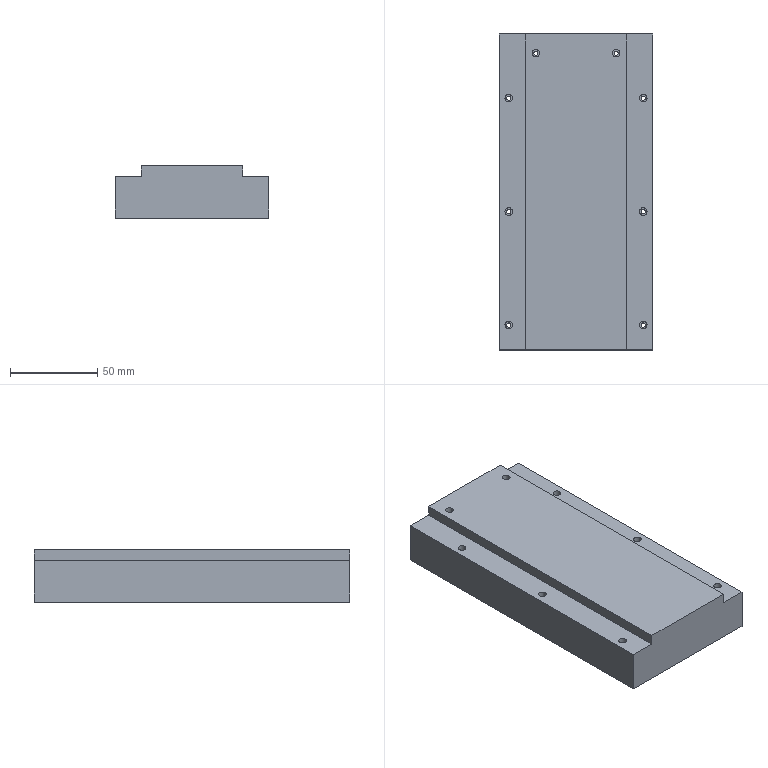NC program | NX | posted with a generic post | part box 88 x 181.05 x 30 mm
Whole program:
N10 G17 G21 G94 G90
(PLANAR_MILL_14 , TOOL : D3-9-D4-50-3T-FINISH)
N12 T10 M6
N14 G54
N16 G17 G0 G90 X-78.489 Y-39.226 B0. C0. S4500 M3
N18 G43 Z60. H10
N20 Z12.
N22 G94 G3 X-78.489 Y-39.226 Z11.753 I0.189 J0.726 F600.
N24 X-78.489 Y-39.226 Z11.506 I0.189 J0.726
N26 X-78.489 Y-39.226 Z11.259 I0.189 J0.726
N28 X-78.489 Y-39.226 Z11.012 I0.189 J0.726
N30 X-78.489 Y-39.226 Z10.765 I0.189 J0.726
N32 X-78.489 Y-39.226 Z10.518 I0.189 J0.726
N34 X-78.489 Y-39.226 Z10.271 I0.189 J0.726
N36 X-78.489 Y-39.226 Z10.024 I0.189 J0.726
N38 X-78.489 Y-39.226 Z9.777 I0.189 J0.726
N40 X-78.489 Y-39.226 Z9.53 I0.189 J0.726
N42 X-78.489 Y-39.226 Z9.283 I0.189 J0.726
N44 X-78.489 Y-39.226 Z9.036 I0.189 J0.726
N46 X-78.489 Y-39.226 Z8.789 I0.189 J0.726
N48 X-78.489 Y-39.226 Z8.542 I0.189 J0.726
N50 X-78.489 Y-39.226 Z8.296 I0.189 J0.726
N52 X-78.489 Y-39.226 Z8.049 I0.189 J0.726
N54 X-78.489 Y-39.226 Z7.802 I0.189 J0.726
N56 X-78.489 Y-39.226 Z7.555 I0.189 J0.726
N58 X-78.489 Y-39.226 Z7.308 I0.189 J0.726
N60 X-78.489 Y-39.226 Z7.061 I0.189 J0.726
N62 X-78.489 Y-39.226 Z6.814 I0.189 J0.726
N64 X-78.489 Y-39.226 Z6.567 I0.189 J0.726
N66 X-78.489 Y-39.226 Z6.32 I0.189 J0.726
N68 X-78.489 Y-39.226 Z6.073 I0.189 J0.726
N70 X-78.489 Y-39.226 Z5.826 I0.189 J0.726
N72 X-78.489 Y-39.226 Z5.579 I0.189 J0.726
N74 X-78.489 Y-39.226 Z5.332 I0.189 J0.726
N76 X-78.489 Y-39.226 Z5.085 I0.189 J0.726
N78 X-78.489 Y-39.226 Z4.838 I0.189 J0.726
N80 X-78.489 Y-39.226 Z4.591 I0.189 J0.726
N82 X-78.489 Y-39.226 Z4.344 I0.189 J0.726
N84 X-78.489 Y-39.226 Z4.097 I0.189 J0.726
N86 X-78.489 Y-39.226 Z3.85 I0.189 J0.726
N88 X-78.489 Y-39.226 Z3.603 I0.189 J0.726
N90 X-78.489 Y-39.226 Z3.356 I0.189 J0.726
N92 X-78.489 Y-39.226 Z3.109 I0.189 J0.726
N94 X-78.489 Y-39.226 Z2.862 I0.189 J0.726
N96 X-78.489 Y-39.226 Z2.615 I0.189 J0.726
N98 X-78.489 Y-39.226 Z2.368 I0.189 J0.726
N100 X-78.489 Y-39.226 Z2.121 I0.189 J0.726
N102 X-78.489 Y-39.226 Z1.874 I0.189 J0.726
N104 X-78.489 Y-39.226 Z1.627 I0.189 J0.726
N106 X-78.489 Y-39.226 Z1.38 I0.189 J0.726
N108 X-78.489 Y-39.226 Z1.134 I0.189 J0.726
N110 X-78.3 Y-37.75 Z1. R-0.75
N112 X-79.05 Y-38.5 R0.75
N114 X-78.3 Y-37.75 R-0.75
N116 G1 Y-39.25
N118 Z4.
N120 G0 Z60.
N122 X-143.111 Y-37.774
N124 Z12.
N126 G3 X-143.111 Y-37.774 Z11.753 I-0.189 J-0.726
N128 X-143.111 Y-37.774 Z11.506 I-0.189 J-0.726
N130 X-143.111 Y-37.774 Z11.259 I-0.189 J-0.726
N132 X-143.111 Y-37.774 Z11.012 I-0.189 J-0.726
N134 X-143.111 Y-37.774 Z10.765 I-0.189 J-0.726
N136 X-143.111 Y-37.774 Z10.518 I-0.189 J-0.726
N138 X-143.111 Y-37.774 Z10.271 I-0.189 J-0.726
N140 X-143.111 Y-37.774 Z10.024 I-0.189 J-0.726
N142 X-143.111 Y-37.774 Z9.777 I-0.189 J-0.726
N144 X-143.111 Y-37.774 Z9.53 I-0.189 J-0.726
N146 X-143.111 Y-37.774 Z9.283 I-0.189 J-0.726
N148 X-143.111 Y-37.774 Z9.036 I-0.189 J-0.726
N150 X-143.111 Y-37.774 Z8.789 I-0.189 J-0.726
N152 X-143.111 Y-37.774 Z8.542 I-0.189 J-0.726
N154 X-143.111 Y-37.774 Z8.296 I-0.189 J-0.726
N156 X-143.111 Y-37.774 Z8.049 I-0.189 J-0.726
N158 X-143.111 Y-37.774 Z7.802 I-0.189 J-0.726
N160 X-143.111 Y-37.774 Z7.555 I-0.189 J-0.726
N162 X-143.111 Y-37.774 Z7.308 I-0.189 J-0.726
N164 X-143.111 Y-37.774 Z7.061 I-0.189 J-0.726
N166 X-143.111 Y-37.774 Z6.814 I-0.189 J-0.726
N168 X-143.111 Y-37.774 Z6.567 I-0.189 J-0.726
N170 X-143.111 Y-37.774 Z6.32 I-0.189 J-0.726
N172 X-143.111 Y-37.774 Z6.073 I-0.189 J-0.726
N174 X-143.111 Y-37.774 Z5.826 I-0.189 J-0.726
N176 X-143.111 Y-37.774 Z5.579 I-0.189 J-0.726
N178 X-143.111 Y-37.774 Z5.332 I-0.189 J-0.726
N180 X-143.111 Y-37.774 Z5.085 I-0.189 J-0.726
N182 X-143.111 Y-37.774 Z4.838 I-0.189 J-0.726
N184 X-143.111 Y-37.774 Z4.591 I-0.189 J-0.726
N186 X-143.111 Y-37.774 Z4.344 I-0.189 J-0.726
N188 X-143.111 Y-37.774 Z4.097 I-0.189 J-0.726
N190 X-143.111 Y-37.774 Z3.85 I-0.189 J-0.726
N192 X-143.111 Y-37.774 Z3.603 I-0.189 J-0.726
N194 X-143.111 Y-37.774 Z3.356 I-0.189 J-0.726
N196 X-143.111 Y-37.774 Z3.109 I-0.189 J-0.726
N198 X-143.111 Y-37.774 Z2.862 I-0.189 J-0.726
N200 X-143.111 Y-37.774 Z2.615 I-0.189 J-0.726
N202 X-143.111 Y-37.774 Z2.368 I-0.189 J-0.726
N204 X-143.111 Y-37.774 Z2.121 I-0.189 J-0.726
N206 X-143.111 Y-37.774 Z1.874 I-0.189 J-0.726
N208 X-143.111 Y-37.774 Z1.627 I-0.189 J-0.726
N210 X-143.111 Y-37.774 Z1.38 I-0.189 J-0.726
N212 X-143.111 Y-37.774 Z1.134 I-0.189 J-0.726
N214 X-143.3 Y-39.25 Z1. R-0.75
N216 X-142.55 Y-38.5 R0.75
N218 X-143.3 Y-39.25 R-0.75
N220 G1 Y-37.75
N222 Z4.
N224 G0 Z60.
N226 X-143.111 Y39.226
N228 Z12.
N230 G3 X-143.111 Y39.226 Z11.753 I-0.189 J-0.726
N232 X-143.111 Y39.226 Z11.506 I-0.189 J-0.726
N234 X-143.111 Y39.226 Z11.259 I-0.189 J-0.726
N236 X-143.111 Y39.226 Z11.012 I-0.189 J-0.726
N238 X-143.111 Y39.226 Z10.765 I-0.189 J-0.726
N240 X-143.111 Y39.226 Z10.518 I-0.189 J-0.726
N242 X-143.111 Y39.226 Z10.271 I-0.189 J-0.726
N244 X-143.111 Y39.226 Z10.024 I-0.189 J-0.726
N246 X-143.111 Y39.226 Z9.777 I-0.189 J-0.726
N248 X-143.111 Y39.226 Z9.53 I-0.189 J-0.726
N250 X-143.111 Y39.226 Z9.283 I-0.189 J-0.726
N252 X-143.111 Y39.226 Z9.036 I-0.189 J-0.726
N254 X-143.111 Y39.226 Z8.789 I-0.189 J-0.726
N256 X-143.111 Y39.226 Z8.542 I-0.189 J-0.726
N258 X-143.111 Y39.226 Z8.296 I-0.189 J-0.726
N260 X-143.111 Y39.226 Z8.049 I-0.189 J-0.726
N262 X-143.111 Y39.226 Z7.802 I-0.189 J-0.726
N264 X-143.111 Y39.226 Z7.555 I-0.189 J-0.726
N266 X-143.111 Y39.226 Z7.308 I-0.189 J-0.726
N268 X-143.111 Y39.226 Z7.061 I-0.189 J-0.726
N270 X-143.111 Y39.226 Z6.814 I-0.189 J-0.726
N272 X-143.111 Y39.226 Z6.567 I-0.189 J-0.726
N274 X-143.111 Y39.226 Z6.32 I-0.189 J-0.726
N276 X-143.111 Y39.226 Z6.073 I-0.189 J-0.726
N278 X-143.111 Y39.226 Z5.826 I-0.189 J-0.726
N280 X-143.111 Y39.226 Z5.579 I-0.189 J-0.726
N282 X-143.111 Y39.226 Z5.332 I-0.189 J-0.726
N284 X-143.111 Y39.226 Z5.085 I-0.189 J-0.726
N286 X-143.111 Y39.226 Z4.838 I-0.189 J-0.726
N288 X-143.111 Y39.226 Z4.591 I-0.189 J-0.726
N290 X-143.111 Y39.226 Z4.344 I-0.189 J-0.726
N292 X-143.111 Y39.226 Z4.097 I-0.189 J-0.726
N294 X-143.111 Y39.226 Z3.85 I-0.189 J-0.726
N296 X-143.111 Y39.226 Z3.603 I-0.189 J-0.726
N298 X-143.111 Y39.226 Z3.356 I-0.189 J-0.726
N300 X-143.111 Y39.226 Z3.109 I-0.189 J-0.726
N302 X-143.111 Y39.226 Z2.862 I-0.189 J-0.726
N304 X-143.111 Y39.226 Z2.615 I-0.189 J-0.726
N306 X-143.111 Y39.226 Z2.368 I-0.189 J-0.726
N308 X-143.111 Y39.226 Z2.121 I-0.189 J-0.726
N310 X-143.111 Y39.226 Z1.874 I-0.189 J-0.726
N312 X-143.111 Y39.226 Z1.627 I-0.189 J-0.726
N314 X-143.111 Y39.226 Z1.38 I-0.189 J-0.726
N316 X-143.111 Y39.226 Z1.134 I-0.189 J-0.726
N318 X-143.3 Y37.75 Z1. R-0.75
N320 X-142.55 Y38.5 R0.75
N322 X-143.3 Y37.75 R-0.75
N324 G1 Y39.25
N326 Z4.
N328 G0 Z60.
N330 X-78.111 Y39.226
N332 Z12.
N334 G3 X-78.111 Y39.226 Z11.753 I-0.189 J-0.726
N336 X-78.111 Y39.226 Z11.506 I-0.189 J-0.726
N338 X-78.111 Y39.226 Z11.259 I-0.189 J-0.726
N340 X-78.111 Y39.226 Z11.012 I-0.189 J-0.726
N342 X-78.111 Y39.226 Z10.765 I-0.189 J-0.726
N344 X-78.111 Y39.226 Z10.518 I-0.189 J-0.726
N346 X-78.111 Y39.226 Z10.271 I-0.189 J-0.726
N348 X-78.111 Y39.226 Z10.024 I-0.189 J-0.726
N350 X-78.111 Y39.226 Z9.777 I-0.189 J-0.726
N352 X-78.111 Y39.226 Z9.53 I-0.189 J-0.726
N354 X-78.111 Y39.226 Z9.283 I-0.189 J-0.726
N356 X-78.111 Y39.226 Z9.036 I-0.189 J-0.726
N358 X-78.111 Y39.226 Z8.789 I-0.189 J-0.726
N360 X-78.111 Y39.226 Z8.542 I-0.189 J-0.726
N362 X-78.111 Y39.226 Z8.296 I-0.189 J-0.726
N364 X-78.111 Y39.226 Z8.049 I-0.189 J-0.726
N366 X-78.111 Y39.226 Z7.802 I-0.189 J-0.726
N368 X-78.111 Y39.226 Z7.555 I-0.189 J-0.726
N370 X-78.111 Y39.226 Z7.308 I-0.189 J-0.726
N372 X-78.111 Y39.226 Z7.061 I-0.189 J-0.726
N374 X-78.111 Y39.226 Z6.814 I-0.189 J-0.726
N376 X-78.111 Y39.226 Z6.567 I-0.189 J-0.726
N378 X-78.111 Y39.226 Z6.32 I-0.189 J-0.726
N380 X-78.111 Y39.226 Z6.073 I-0.189 J-0.726
N382 X-78.111 Y39.226 Z5.826 I-0.189 J-0.726
N384 X-78.111 Y39.226 Z5.579 I-0.189 J-0.726
N386 X-78.111 Y39.226 Z5.332 I-0.189 J-0.726
N388 X-78.111 Y39.226 Z5.085 I-0.189 J-0.726
N390 X-78.111 Y39.226 Z4.838 I-0.189 J-0.726
N392 X-78.111 Y39.226 Z4.591 I-0.189 J-0.726
N394 X-78.111 Y39.226 Z4.344 I-0.189 J-0.726
N396 X-78.111 Y39.226 Z4.097 I-0.189 J-0.726
N398 X-78.111 Y39.226 Z3.85 I-0.189 J-0.726
N400 X-78.111 Y39.226 Z3.603 I-0.189 J-0.726
N402 X-78.111 Y39.226 Z3.356 I-0.189 J-0.726
N404 X-78.111 Y39.226 Z3.109 I-0.189 J-0.726
N406 X-78.111 Y39.226 Z2.862 I-0.189 J-0.726
N408 X-78.111 Y39.226 Z2.615 I-0.189 J-0.726
N410 X-78.111 Y39.226 Z2.368 I-0.189 J-0.726
N412 X-78.111 Y39.226 Z2.121 I-0.189 J-0.726
N414 X-78.111 Y39.226 Z1.874 I-0.189 J-0.726
N416 X-78.111 Y39.226 Z1.627 I-0.189 J-0.726
N418 X-78.111 Y39.226 Z1.38 I-0.189 J-0.726
N420 X-78.111 Y39.226 Z1.134 I-0.189 J-0.726
N422 X-78.3 Y37.75 Z1. R-0.75
N424 X-77.55 Y38.5 R0.75
N426 X-78.3 Y37.75 R-0.75
N428 G1 Y39.25
N430 Z4.
N432 G0 Z60.
(PLANAR_MILL_14_COPY , TOOL : D3-9-D4-50-3T-FINISH)
N434 X-169.547 Y23.561
N436 Z19.
N438 G3 X-169.547 Y23.561 Z18.753 I0.497 J-0.561
N440 X-169.547 Y23.561 Z18.506 I0.497 J-0.561
N442 X-169.547 Y23.561 Z18.259 I0.497 J-0.561
N444 X-169.547 Y23.561 Z18.012 I0.497 J-0.561
N446 X-169.547 Y23.561 Z17.765 I0.497 J-0.561
N448 X-169.547 Y23.561 Z17.518 I0.497 J-0.561
N450 X-169.547 Y23.561 Z17.271 I0.497 J-0.561
N452 X-169.547 Y23.561 Z17.024 I0.497 J-0.561
N454 X-169.547 Y23.561 Z16.777 I0.497 J-0.561
N456 X-169.547 Y23.561 Z16.53 I0.497 J-0.561
N458 X-169.547 Y23.561 Z16.283 I0.497 J-0.561
N460 X-169.547 Y23.561 Z16.036 I0.497 J-0.561
N462 X-169.547 Y23.561 Z15.789 I0.497 J-0.561
N464 X-169.547 Y23.561 Z15.542 I0.497 J-0.561
N466 X-169.547 Y23.561 Z15.296 I0.497 J-0.561
N468 X-169.547 Y23.561 Z15.049 I0.497 J-0.561
N470 X-169.547 Y23.561 Z14.802 I0.497 J-0.561
N472 X-169.547 Y23.561 Z14.555 I0.497 J-0.561
N474 X-169.547 Y23.561 Z14.308 I0.497 J-0.561
N476 X-169.547 Y23.561 Z14.061 I0.497 J-0.561
N478 X-169.547 Y23.561 Z13.814 I0.497 J-0.561
N480 X-169.547 Y23.561 Z13.567 I0.497 J-0.561
N482 X-169.547 Y23.561 Z13.32 I0.497 J-0.561
N484 X-169.547 Y23.561 Z13.073 I0.497 J-0.561
N486 X-169.547 Y23.561 Z12.826 I0.497 J-0.561
N488 X-169.547 Y23.561 Z12.579 I0.497 J-0.561
N490 X-169.547 Y23.561 Z12.332 I0.497 J-0.561
N492 X-169.547 Y23.561 Z12.085 I0.497 J-0.561
N494 X-169.547 Y23.561 Z11.838 I0.497 J-0.561
N496 X-169.547 Y23.561 Z11.591 I0.497 J-0.561
N498 X-169.547 Y23.561 Z11.344 I0.497 J-0.561
N500 X-169.547 Y23.561 Z11.097 I0.497 J-0.561
N502 X-169.547 Y23.561 Z10.85 I0.497 J-0.561
N504 X-169.547 Y23.561 Z10.603 I0.497 J-0.561
N506 X-169.547 Y23.561 Z10.356 I0.497 J-0.561
N508 X-169.547 Y23.561 Z10.109 I0.497 J-0.561
N510 X-169.547 Y23.561 Z9.862 I0.497 J-0.561
N512 X-169.547 Y23.561 Z9.615 I0.497 J-0.561
N514 X-169.547 Y23.561 Z9.368 I0.497 J-0.561
N516 X-169.547 Y23.561 Z9.121 I0.497 J-0.561
N518 X-169.547 Y23.561 Z8.874 I0.497 J-0.561
N520 X-169.547 Y23.561 Z8.627 I0.497 J-0.561
N522 X-169.547 Y23.561 Z8.38 I0.497 J-0.561
N524 X-169.547 Y23.561 Z8.134 I0.497 J-0.561
N526 X-169.547 Y23.561 Z7.887 I0.497 J-0.561
N528 X-169.547 Y23.561 Z7.64 I0.497 J-0.561
N530 X-169.547 Y23.561 Z7.393 I0.497 J-0.561
N532 X-169.547 Y23.561 Z7.146 I0.497 J-0.561
N534 X-169.547 Y23.561 Z6.899 I0.497 J-0.561
N536 X-169.547 Y23.561 Z6.652 I0.497 J-0.561
N538 X-169.547 Y23.561 Z6.405 I0.497 J-0.561
N540 X-169.547 Y23.561 Z6.158 I0.497 J-0.561
N542 X-169.547 Y23.561 Z5.911 I0.497 J-0.561
N544 X-169.547 Y23.561 Z5.664 I0.497 J-0.561
N546 X-169.547 Y23.561 Z5.417 I0.497 J-0.561
N548 X-169.547 Y23.561 Z5.17 I0.497 J-0.561
N550 X-169.547 Y23.561 Z4.923 I0.497 J-0.561
N552 X-169.547 Y23.561 Z4.676 I0.497 J-0.561
N554 X-169.547 Y23.561 Z4.429 I0.497 J-0.561
N556 X-169.547 Y23.561 Z4.182 I0.497 J-0.561
N558 X-169.547 Y23.561 Z3.935 I0.497 J-0.561
N560 X-169.547 Y23.561 Z3.688 I0.497 J-0.561
N562 X-169.547 Y23.561 Z3.441 I0.497 J-0.561
N564 X-169.547 Y23.561 Z3.194 I0.497 J-0.561
N566 X-169.547 Y23.561 Z2.947 I0.497 J-0.561
N568 X-169.547 Y23.561 Z2.7 I0.497 J-0.561
N570 X-169.547 Y23.561 Z2.453 I0.497 J-0.561
N572 X-169.547 Y23.561 Z2.206 I0.497 J-0.561
N574 X-169.547 Y23.561 Z1.959 I0.497 J-0.561
N576 X-169.547 Y23.561 Z1.712 I0.497 J-0.561
N578 X-169.547 Y23.561 Z1.465 I0.497 J-0.561
N580 X-169.547 Y23.561 Z1.218 I0.497 J-0.561
N582 X-169.05 Y23.75 Z1. R-0.75
N584 X-169.8 Y23. R0.75
N586 X-169.05 Y23.75 R-0.75
N588 G1 Z2.
N590 G0 Z60.
N592 X-169.547 Y-22.439
N594 Z19.
N596 G3 X-169.547 Y-22.439 Z18.753 I0.497 J-0.561
N598 X-169.547 Y-22.439 Z18.506 I0.497 J-0.561
N600 X-169.547 Y-22.439 Z18.259 I0.497 J-0.561
N602 X-169.547 Y-22.439 Z18.012 I0.497 J-0.561
N604 X-169.547 Y-22.439 Z17.765 I0.497 J-0.561
N606 X-169.547 Y-22.439 Z17.518 I0.497 J-0.561
N608 X-169.547 Y-22.439 Z17.271 I0.497 J-0.561
N610 X-169.547 Y-22.439 Z17.024 I0.497 J-0.561
N612 X-169.547 Y-22.439 Z16.777 I0.497 J-0.561
N614 X-169.547 Y-22.439 Z16.53 I0.497 J-0.561
N616 X-169.547 Y-22.439 Z16.283 I0.497 J-0.561
N618 X-169.547 Y-22.439 Z16.036 I0.497 J-0.561
N620 X-169.547 Y-22.439 Z15.789 I0.497 J-0.561
N622 X-169.547 Y-22.439 Z15.542 I0.497 J-0.561
N624 X-169.547 Y-22.439 Z15.296 I0.497 J-0.561
N626 X-169.547 Y-22.439 Z15.049 I0.497 J-0.561
N628 X-169.547 Y-22.439 Z14.802 I0.497 J-0.561
N630 X-169.547 Y-22.439 Z14.555 I0.497 J-0.561
N632 X-169.547 Y-22.439 Z14.308 I0.497 J-0.561
N634 X-169.547 Y-22.439 Z14.061 I0.497 J-0.561
N636 X-169.547 Y-22.439 Z13.814 I0.497 J-0.561
N638 X-169.547 Y-22.439 Z13.567 I0.497 J-0.561
N640 X-169.547 Y-22.439 Z13.32 I0.497 J-0.561
N642 X-169.547 Y-22.439 Z13.073 I0.497 J-0.561
N644 X-169.547 Y-22.439 Z12.826 I0.497 J-0.561
N646 X-169.547 Y-22.439 Z12.579 I0.497 J-0.561
N648 X-169.547 Y-22.439 Z12.332 I0.497 J-0.561
N650 X-169.547 Y-22.439 Z12.085 I0.497 J-0.561
N652 X-169.547 Y-22.439 Z11.838 I0.497 J-0.561
N654 X-169.547 Y-22.439 Z11.591 I0.497 J-0.561
N656 X-169.547 Y-22.439 Z11.344 I0.497 J-0.561
N658 X-169.547 Y-22.439 Z11.097 I0.497 J-0.561
N660 X-169.547 Y-22.439 Z10.85 I0.497 J-0.561
N662 X-169.547 Y-22.439 Z10.603 I0.497 J-0.561
N664 X-169.547 Y-22.439 Z10.356 I0.497 J-0.561
N666 X-169.547 Y-22.439 Z10.109 I0.497 J-0.561
N668 X-169.547 Y-22.439 Z9.862 I0.497 J-0.561
N670 X-169.547 Y-22.439 Z9.615 I0.497 J-0.561
N672 X-169.547 Y-22.439 Z9.368 I0.497 J-0.561
N674 X-169.547 Y-22.439 Z9.121 I0.497 J-0.561
N676 X-169.547 Y-22.439 Z8.874 I0.497 J-0.561
N678 X-169.547 Y-22.439 Z8.627 I0.497 J-0.561
N680 X-169.547 Y-22.439 Z8.38 I0.497 J-0.561
N682 X-169.547 Y-22.439 Z8.134 I0.497 J-0.561
N684 X-169.547 Y-22.439 Z7.887 I0.497 J-0.561
N686 X-169.547 Y-22.439 Z7.64 I0.497 J-0.561
N688 X-169.547 Y-22.439 Z7.393 I0.497 J-0.561
N690 X-169.547 Y-22.439 Z7.146 I0.497 J-0.561
N692 X-169.547 Y-22.439 Z6.899 I0.497 J-0.561
N694 X-169.547 Y-22.439 Z6.652 I0.497 J-0.561
N696 X-169.547 Y-22.439 Z6.405 I0.497 J-0.561
N698 X-169.547 Y-22.439 Z6.158 I0.497 J-0.561
N700 X-169.547 Y-22.439 Z5.911 I0.497 J-0.561
N702 X-169.547 Y-22.439 Z5.664 I0.497 J-0.561
N704 X-169.547 Y-22.439 Z5.417 I0.497 J-0.561
N706 X-169.547 Y-22.439 Z5.17 I0.497 J-0.561
N708 X-169.547 Y-22.439 Z4.923 I0.497 J-0.561
N710 X-169.547 Y-22.439 Z4.676 I0.497 J-0.561
N712 X-169.547 Y-22.439 Z4.429 I0.497 J-0.561
N714 X-169.547 Y-22.439 Z4.182 I0.497 J-0.561
N716 X-169.547 Y-22.439 Z3.935 I0.497 J-0.561
N718 X-169.547 Y-22.439 Z3.688 I0.497 J-0.561
N720 X-169.547 Y-22.439 Z3.441 I0.497 J-0.561
N722 X-169.547 Y-22.439 Z3.194 I0.497 J-0.561
N724 X-169.547 Y-22.439 Z2.947 I0.497 J-0.561
N726 X-169.547 Y-22.439 Z2.7 I0.497 J-0.561
N728 X-169.547 Y-22.439 Z2.453 I0.497 J-0.561
N730 X-169.547 Y-22.439 Z2.206 I0.497 J-0.561
N732 X-169.547 Y-22.439 Z1.959 I0.497 J-0.561
N734 X-169.547 Y-22.439 Z1.712 I0.497 J-0.561
N736 X-169.547 Y-22.439 Z1.465 I0.497 J-0.561
N738 X-169.547 Y-22.439 Z1.218 I0.497 J-0.561
N740 X-169.05 Y-22.25 Z1. R-0.75
N742 X-169.8 Y-23. R0.75
N744 X-169.05 Y-22.25 R-0.75
N746 G1 Z2.
N748 G0 Z60.
(PLANAR_MILL_14_COPY_COPY , TOOL : D3-9-D4-50-3T-FINISH)
N750 X-12.592 Y38.747
N752 Z5.
N754 G3 X-12.592 Y38.747 Z4.753 I-0.708 J-0.247
N756 X-12.592 Y38.747 Z4.506 I-0.708 J-0.247
N758 X-12.592 Y38.747 Z4.259 I-0.708 J-0.247
N760 X-12.592 Y38.747 Z4.012 I-0.708 J-0.247
N762 X-12.592 Y38.747 Z3.765 I-0.708 J-0.247
N764 X-12.592 Y38.747 Z3.518 I-0.708 J-0.247
N766 X-12.592 Y38.747 Z3.271 I-0.708 J-0.247
N768 X-12.592 Y38.747 Z3.024 I-0.708 J-0.247
N770 X-12.592 Y38.747 Z2.777 I-0.708 J-0.247
N772 X-12.592 Y38.747 Z2.53 I-0.708 J-0.247
N774 X-12.592 Y38.747 Z2.283 I-0.708 J-0.247
N776 X-12.592 Y38.747 Z2.036 I-0.708 J-0.247
N778 X-12.592 Y38.747 Z1.789 I-0.708 J-0.247
N780 X-12.592 Y38.747 Z1.542 I-0.708 J-0.247
N782 X-12.592 Y38.747 Z1.296 I-0.708 J-0.247
N784 X-12.592 Y38.747 Z1.049 I-0.708 J-0.247
N786 X-13.3 Y39.25 Z1. R0.75
N788 X-14.05 Y38.5 R0.75
N790 X-13.3 Y39.25 R-0.75
N792 G1 Z2.
N794 G0 Z60.
N796 X-12.592 Y-38.253
N798 Z5.
N800 G3 X-12.592 Y-38.253 Z4.753 I-0.708 J-0.247
N802 X-12.592 Y-38.253 Z4.506 I-0.708 J-0.247
N804 X-12.592 Y-38.253 Z4.259 I-0.708 J-0.247
N806 X-12.592 Y-38.253 Z4.012 I-0.708 J-0.247
N808 X-12.592 Y-38.253 Z3.765 I-0.708 J-0.247
N810 X-12.592 Y-38.253 Z3.518 I-0.708 J-0.247
N812 X-12.592 Y-38.253 Z3.271 I-0.708 J-0.247
N814 X-12.592 Y-38.253 Z3.024 I-0.708 J-0.247
N816 X-12.592 Y-38.253 Z2.777 I-0.708 J-0.247
N818 X-12.592 Y-38.253 Z2.53 I-0.708 J-0.247
N820 X-12.592 Y-38.253 Z2.283 I-0.708 J-0.247
N822 X-12.592 Y-38.253 Z2.036 I-0.708 J-0.247
N824 X-12.592 Y-38.253 Z1.789 I-0.708 J-0.247
N826 X-12.592 Y-38.253 Z1.542 I-0.708 J-0.247
N828 X-12.592 Y-38.253 Z1.296 I-0.708 J-0.247
N830 X-12.592 Y-38.253 Z1.049 I-0.708 J-0.247
N832 X-13.3 Y-37.75 Z1. R0.75
N834 X-14.05 Y-38.5 R0.75
N836 X-13.3 Y-37.75 R-0.75
N838 G1 Z2.
N840 G0 Z60.
N842 M5
N844 M2